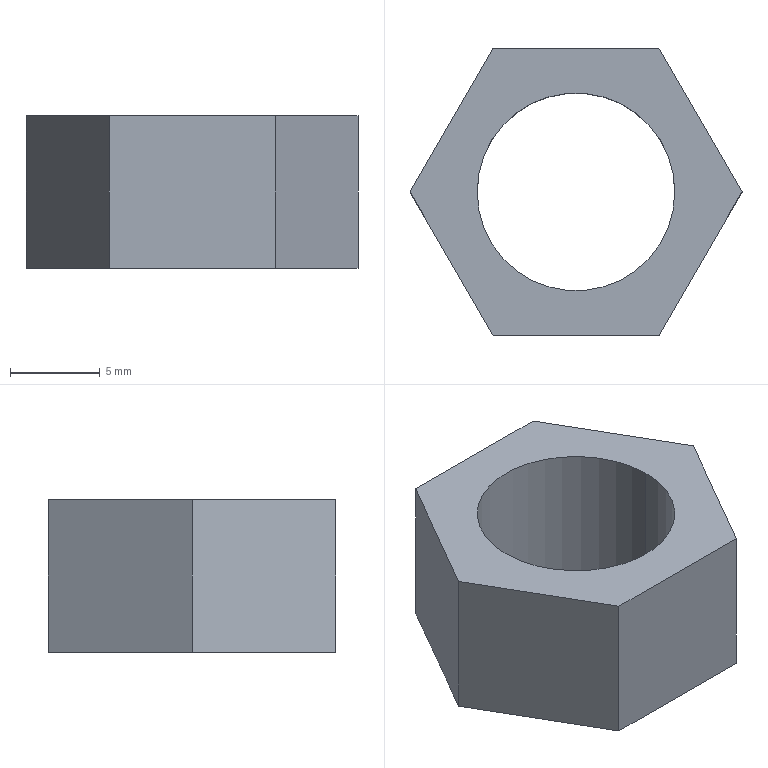Part | SolidWorks | features Extrusion 1, ICE 1 | 1 solid | 10 faces | box 18.475 x 16 x 8.5 mm | volume 1077 mm3 | plane 8 | cylinder 2 | commonest cylinder face diameters 11 x2
STEP:
#1=CARTESIAN_POINT('',(-5.5,0.,0.));
#2=VERTEX_POINT('',#1);
#3=CARTESIAN_POINT('',(5.5,0.,0.));
#4=VERTEX_POINT('',#3);
#5=CARTESIAN_POINT('',(0.,0.,0.));
#6=DIRECTION('',(0.,0.,1.));
#7=DIRECTION('',(1.,0.,0.));
#8=AXIS2_PLACEMENT_3D('',#5,#6,#7);
#9=CIRCLE('',#8,5.5);
#10=EDGE_CURVE('',#2,#4,#9,.T.);
#11=ORIENTED_EDGE('',*,*,#10,.F.);
#12=CARTESIAN_POINT('',(-5.5,0.,8.5));
#13=VERTEX_POINT('',#12);
#14=CARTESIAN_POINT('',(-5.5,0.,0.));
#15=DIRECTION('',(0.,0.,1.));
#16=VECTOR('',#15,1000.);
#17=LINE('',#14,#16);
#18=EDGE_CURVE('',#2,#13,#17,.T.);
#19=ORIENTED_EDGE('',*,*,#18,.T.);
#20=CARTESIAN_POINT('',(5.5,0.,8.5));
#21=VERTEX_POINT('',#20);
#22=CARTESIAN_POINT('',(0.,0.,8.5));
#23=DIRECTION('',(0.,0.,1.));
#24=DIRECTION('',(1.,0.,0.));
#25=AXIS2_PLACEMENT_3D('',#22,#23,#24);
#26=CIRCLE('',#25,5.5);
#27=EDGE_CURVE('',#13,#21,#26,.T.);
#28=ORIENTED_EDGE('',*,*,#27,.T.);
#29=CARTESIAN_POINT('',(5.5,0.,0.));
#30=DIRECTION('',(0.,0.,1.));
#31=VECTOR('',#30,1000.);
#32=LINE('',#29,#31);
#33=EDGE_CURVE('',#4,#21,#32,.T.);
#34=ORIENTED_EDGE('',*,*,#33,.F.);
#35=EDGE_LOOP('',(#11,#19,#28,#34));
#36=FACE_OUTER_BOUND('',#35,.T.);
#37=CARTESIAN_POINT('',(0.,0.,0.));
#38=DIRECTION('',(0.,0.,1.));
#39=DIRECTION('',(1.,0.,0.));
#40=AXIS2_PLACEMENT_3D('',#37,#38,#39);
#41=CYLINDRICAL_SURFACE('',#40,5.5);
#42=ADVANCED_FACE('',(#36),#41,.F.);
#43=CARTESIAN_POINT('',(4.619,-8.,0.));
#44=VERTEX_POINT('',#43);
#45=CARTESIAN_POINT('',(9.238,0.,0.));
#46=VERTEX_POINT('',#45);
#47=CARTESIAN_POINT('',(4.619,-8.,0.));
#48=DIRECTION('',(0.5,0.866,0.));
#49=VECTOR('',#48,1000.);
#50=LINE('',#47,#49);
#51=EDGE_CURVE('',#44,#46,#50,.T.);
#52=ORIENTED_EDGE('',*,*,#51,.T.);
#53=CARTESIAN_POINT('',(9.238,0.,8.5));
#54=VERTEX_POINT('',#53);
#55=CARTESIAN_POINT('',(9.238,0.,8.5));
#56=DIRECTION('',(0.,0.,-1.));
#57=VECTOR('',#56,1000.);
#58=LINE('',#55,#57);
#59=EDGE_CURVE('',#54,#46,#58,.T.);
#60=ORIENTED_EDGE('',*,*,#59,.F.);
#61=CARTESIAN_POINT('',(4.619,-8.,8.5));
#62=VERTEX_POINT('',#61);
#63=CARTESIAN_POINT('',(4.619,-8.,8.5));
#64=DIRECTION('',(0.5,0.866,0.));
#65=VECTOR('',#64,1000.);
#66=LINE('',#63,#65);
#67=EDGE_CURVE('',#62,#54,#66,.T.);
#68=ORIENTED_EDGE('',*,*,#67,.F.);
#69=CARTESIAN_POINT('',(4.619,-8.,8.5));
#70=DIRECTION('',(0.,0.,-1.));
#71=VECTOR('',#70,1000.);
#72=LINE('',#69,#71);
#73=EDGE_CURVE('',#62,#44,#72,.T.);
#74=ORIENTED_EDGE('',*,*,#73,.T.);
#75=EDGE_LOOP('',(#52,#60,#68,#74));
#76=FACE_OUTER_BOUND('',#75,.T.);
#77=CARTESIAN_POINT('',(4.619,-8.,8.5));
#78=DIRECTION('',(-0.866,0.5,0.));
#79=DIRECTION('',(-0.5,-0.866,0.));
#80=AXIS2_PLACEMENT_3D('',#77,#78,#79);
#81=PLANE('',#80);
#82=ADVANCED_FACE('',(#76),#81,.F.);
#83=CARTESIAN_POINT('',(4.619,8.,0.));
#84=VERTEX_POINT('',#83);
#85=CARTESIAN_POINT('',(9.238,0.,0.));
#86=DIRECTION('',(-0.5,0.866,0.));
#87=VECTOR('',#86,1000.);
#88=LINE('',#85,#87);
#89=EDGE_CURVE('',#46,#84,#88,.T.);
#90=ORIENTED_EDGE('',*,*,#89,.T.);
#91=CARTESIAN_POINT('',(4.619,8.,8.5));
#92=VERTEX_POINT('',#91);
#93=CARTESIAN_POINT('',(4.619,8.,8.5));
#94=DIRECTION('',(0.,0.,-1.));
#95=VECTOR('',#94,1000.);
#96=LINE('',#93,#95);
#97=EDGE_CURVE('',#92,#84,#96,.T.);
#98=ORIENTED_EDGE('',*,*,#97,.F.);
#99=CARTESIAN_POINT('',(9.238,0.,8.5));
#100=DIRECTION('',(-0.5,0.866,0.));
#101=VECTOR('',#100,1000.);
#102=LINE('',#99,#101);
#103=EDGE_CURVE('',#54,#92,#102,.T.);
#104=ORIENTED_EDGE('',*,*,#103,.F.);
#105=ORIENTED_EDGE('',*,*,#59,.T.);
#106=EDGE_LOOP('',(#90,#98,#104,#105));
#107=FACE_OUTER_BOUND('',#106,.T.);
#108=CARTESIAN_POINT('',(9.238,0.,8.5));
#109=DIRECTION('',(-0.866,-0.5,0.));
#110=DIRECTION('',(0.5,-0.866,0.));
#111=AXIS2_PLACEMENT_3D('',#108,#109,#110);
#112=PLANE('',#111);
#113=ADVANCED_FACE('',(#107),#112,.F.);
#114=CARTESIAN_POINT('',(-4.619,8.,0.));
#115=VERTEX_POINT('',#114);
#116=CARTESIAN_POINT('',(4.619,8.,0.));
#117=DIRECTION('',(-1.,0.,0.));
#118=VECTOR('',#117,1000.);
#119=LINE('',#116,#118);
#120=EDGE_CURVE('',#84,#115,#119,.T.);
#121=ORIENTED_EDGE('',*,*,#120,.T.);
#122=CARTESIAN_POINT('',(-4.619,8.,8.5));
#123=VERTEX_POINT('',#122);
#124=CARTESIAN_POINT('',(-4.619,8.,8.5));
#125=DIRECTION('',(0.,0.,-1.));
#126=VECTOR('',#125,1000.);
#127=LINE('',#124,#126);
#128=EDGE_CURVE('',#123,#115,#127,.T.);
#129=ORIENTED_EDGE('',*,*,#128,.F.);
#130=CARTESIAN_POINT('',(4.619,8.,8.5));
#131=DIRECTION('',(-1.,0.,0.));
#132=VECTOR('',#131,1000.);
#133=LINE('',#130,#132);
#134=EDGE_CURVE('',#92,#123,#133,.T.);
#135=ORIENTED_EDGE('',*,*,#134,.F.);
#136=ORIENTED_EDGE('',*,*,#97,.T.);
#137=EDGE_LOOP('',(#121,#129,#135,#136));
#138=FACE_OUTER_BOUND('',#137,.T.);
#139=CARTESIAN_POINT('',(4.619,8.,8.5));
#140=DIRECTION('',(0.,-1.,0.));
#141=DIRECTION('',(1.,0.,0.));
#142=AXIS2_PLACEMENT_3D('',#139,#140,#141);
#143=PLANE('',#142);
#144=ADVANCED_FACE('',(#138),#143,.F.);
#145=CARTESIAN_POINT('',(-9.238,0.,0.));
#146=VERTEX_POINT('',#145);
#147=CARTESIAN_POINT('',(-4.619,8.,0.));
#148=DIRECTION('',(-0.5,-0.866,0.));
#149=VECTOR('',#148,1000.);
#150=LINE('',#147,#149);
#151=EDGE_CURVE('',#115,#146,#150,.T.);
#152=ORIENTED_EDGE('',*,*,#151,.T.);
#153=CARTESIAN_POINT('',(-9.238,0.,8.5));
#154=VERTEX_POINT('',#153);
#155=CARTESIAN_POINT('',(-9.238,0.,8.5));
#156=DIRECTION('',(0.,0.,-1.));
#157=VECTOR('',#156,1000.);
#158=LINE('',#155,#157);
#159=EDGE_CURVE('',#154,#146,#158,.T.);
#160=ORIENTED_EDGE('',*,*,#159,.F.);
#161=CARTESIAN_POINT('',(-4.619,8.,8.5));
#162=DIRECTION('',(-0.5,-0.866,0.));
#163=VECTOR('',#162,1000.);
#164=LINE('',#161,#163);
#165=EDGE_CURVE('',#123,#154,#164,.T.);
#166=ORIENTED_EDGE('',*,*,#165,.F.);
#167=ORIENTED_EDGE('',*,*,#128,.T.);
#168=EDGE_LOOP('',(#152,#160,#166,#167));
#169=FACE_OUTER_BOUND('',#168,.T.);
#170=CARTESIAN_POINT('',(-4.619,8.,8.5));
#171=DIRECTION('',(0.866,-0.5,0.));
#172=DIRECTION('',(0.5,0.866,0.));
#173=AXIS2_PLACEMENT_3D('',#170,#171,#172);
#174=PLANE('',#173);
#175=ADVANCED_FACE('',(#169),#174,.F.);
#176=CARTESIAN_POINT('',(-4.619,-8.,0.));
#177=VERTEX_POINT('',#176);
#178=CARTESIAN_POINT('',(-9.238,0.,0.));
#179=DIRECTION('',(0.5,-0.866,0.));
#180=VECTOR('',#179,1000.);
#181=LINE('',#178,#180);
#182=EDGE_CURVE('',#146,#177,#181,.T.);
#183=ORIENTED_EDGE('',*,*,#182,.T.);
#184=CARTESIAN_POINT('',(-4.619,-8.,8.5));
#185=VERTEX_POINT('',#184);
#186=CARTESIAN_POINT('',(-4.619,-8.,8.5));
#187=DIRECTION('',(0.,0.,-1.));
#188=VECTOR('',#187,1000.);
#189=LINE('',#186,#188);
#190=EDGE_CURVE('',#185,#177,#189,.T.);
#191=ORIENTED_EDGE('',*,*,#190,.F.);
#192=CARTESIAN_POINT('',(-9.238,0.,8.5));
#193=DIRECTION('',(0.5,-0.866,0.));
#194=VECTOR('',#193,1000.);
#195=LINE('',#192,#194);
#196=EDGE_CURVE('',#154,#185,#195,.T.);
#197=ORIENTED_EDGE('',*,*,#196,.F.);
#198=ORIENTED_EDGE('',*,*,#159,.T.);
#199=EDGE_LOOP('',(#183,#191,#197,#198));
#200=FACE_OUTER_BOUND('',#199,.T.);
#201=CARTESIAN_POINT('',(-9.238,0.,8.5));
#202=DIRECTION('',(0.866,0.5,0.));
#203=DIRECTION('',(-0.5,0.866,0.));
#204=AXIS2_PLACEMENT_3D('',#201,#202,#203);
#205=PLANE('',#204);
#206=ADVANCED_FACE('',(#200),#205,.F.);
#207=CARTESIAN_POINT('',(-4.619,-8.,0.));
#208=DIRECTION('',(1.,0.,0.));
#209=VECTOR('',#208,1000.);
#210=LINE('',#207,#209);
#211=EDGE_CURVE('',#177,#44,#210,.T.);
#212=ORIENTED_EDGE('',*,*,#211,.T.);
#213=ORIENTED_EDGE('',*,*,#73,.F.);
#214=CARTESIAN_POINT('',(-4.619,-8.,8.5));
#215=DIRECTION('',(1.,0.,0.));
#216=VECTOR('',#215,1000.);
#217=LINE('',#214,#216);
#218=EDGE_CURVE('',#185,#62,#217,.T.);
#219=ORIENTED_EDGE('',*,*,#218,.F.);
#220=ORIENTED_EDGE('',*,*,#190,.T.);
#221=EDGE_LOOP('',(#212,#213,#219,#220));
#222=FACE_OUTER_BOUND('',#221,.T.);
#223=CARTESIAN_POINT('',(-4.619,-8.,8.5));
#224=DIRECTION('',(0.,1.,0.));
#225=DIRECTION('',(-1.,0.,0.));
#226=AXIS2_PLACEMENT_3D('',#223,#224,#225);
#227=PLANE('',#226);
#228=ADVANCED_FACE('',(#222),#227,.F.);
#229=CARTESIAN_POINT('',(0.,0.,8.5));
#230=DIRECTION('',(0.,0.,1.));
#231=DIRECTION('',(1.,0.,0.));
#232=AXIS2_PLACEMENT_3D('',#229,#230,#231);
#233=CIRCLE('',#232,5.5);
#234=EDGE_CURVE('',#21,#13,#233,.T.);
#235=ORIENTED_EDGE('',*,*,#234,.F.);
#236=ORIENTED_EDGE('',*,*,#27,.F.);
#237=EDGE_LOOP('',(#235,#236));
#238=FACE_BOUND('',#237,.T.);
#239=ORIENTED_EDGE('',*,*,#67,.T.);
#240=ORIENTED_EDGE('',*,*,#103,.T.);
#241=ORIENTED_EDGE('',*,*,#134,.T.);
#242=ORIENTED_EDGE('',*,*,#165,.T.);
#243=ORIENTED_EDGE('',*,*,#196,.T.);
#244=ORIENTED_EDGE('',*,*,#218,.T.);
#245=EDGE_LOOP('',(#239,#240,#241,#242,#243,#244));
#246=FACE_OUTER_BOUND('',#245,.T.);
#247=CARTESIAN_POINT('',(0.,0.,8.5));
#248=DIRECTION('',(0.,0.,1.));
#249=DIRECTION('',(1.,0.,0.));
#250=AXIS2_PLACEMENT_3D('',#247,#248,#249);
#251=PLANE('',#250);
#252=ADVANCED_FACE('',(#238,#246),#251,.T.);
#253=CARTESIAN_POINT('',(0.,0.,0.));
#254=DIRECTION('',(0.,0.,1.));
#255=DIRECTION('',(1.,0.,0.));
#256=AXIS2_PLACEMENT_3D('',#253,#254,#255);
#257=CIRCLE('',#256,5.5);
#258=EDGE_CURVE('',#4,#2,#257,.T.);
#259=ORIENTED_EDGE('',*,*,#258,.T.);
#260=ORIENTED_EDGE('',*,*,#10,.T.);
#261=EDGE_LOOP('',(#259,#260));
#262=FACE_BOUND('',#261,.T.);
#263=ORIENTED_EDGE('',*,*,#51,.F.);
#264=ORIENTED_EDGE('',*,*,#211,.F.);
#265=ORIENTED_EDGE('',*,*,#182,.F.);
#266=ORIENTED_EDGE('',*,*,#151,.F.);
#267=ORIENTED_EDGE('',*,*,#120,.F.);
#268=ORIENTED_EDGE('',*,*,#89,.F.);
#269=EDGE_LOOP('',(#263,#264,#265,#266,#267,#268));
#270=FACE_OUTER_BOUND('',#269,.T.);
#271=CARTESIAN_POINT('',(0.,0.,0.));
#272=DIRECTION('',(0.,0.,1.));
#273=DIRECTION('',(1.,0.,0.));
#274=AXIS2_PLACEMENT_3D('',#271,#272,#273);
#275=PLANE('',#274);
#276=ADVANCED_FACE('',(#262,#270),#275,.F.);
#277=ORIENTED_EDGE('',*,*,#18,.F.);
#278=ORIENTED_EDGE('',*,*,#258,.F.);
#279=ORIENTED_EDGE('',*,*,#33,.T.);
#280=ORIENTED_EDGE('',*,*,#234,.T.);
#281=EDGE_LOOP('',(#277,#278,#279,#280));
#282=FACE_OUTER_BOUND('',#281,.T.);
#283=CARTESIAN_POINT('',(0.,0.,0.));
#284=DIRECTION('',(0.,0.,1.));
#285=DIRECTION('',(1.,0.,0.));
#286=AXIS2_PLACEMENT_3D('',#283,#284,#285);
#287=CYLINDRICAL_SURFACE('',#286,5.5);
#288=ADVANCED_FACE('',(#282),#287,.F.);
#289=CLOSED_SHELL('',(#42,#82,#113,#144,#175,#206,#228,#252,#276,#288));
#290=MANIFOLD_SOLID_BREP('',#289);
#291=CARTESIAN_POINT('',(0.,0.,0.));
#292=DIRECTION('',(0.,0.,1.));
#293=DIRECTION('',(1.,0.,0.));
#294=AXIS2_PLACEMENT_3D('',#291,#292,#293);
#295=(LENGTH_UNIT()NAMED_UNIT(*)SI_UNIT(.MILLI.,.METRE.));
#296=UNCERTAINTY_MEASURE_WITH_UNIT(LENGTH_MEASURE(0.00001),#295,'','');
#297=(NAMED_UNIT(*)PLANE_ANGLE_UNIT()SI_UNIT($,.RADIAN.));
#298=(NAMED_UNIT(*)SI_UNIT($,.STERADIAN.)SOLID_ANGLE_UNIT());
#299=(GEOMETRIC_REPRESENTATION_CONTEXT(3)GLOBAL_UNCERTAINTY_ASSIGNED_CONTEXT((#296))GLOBAL_UNIT_ASSIGNED_CONTEXT((#295,#297,#298))REPRESENTATION_CONTEXT('',''));
#300=ADVANCED_BREP_SHAPE_REPRESENTATION('',(#290,#294),#299);